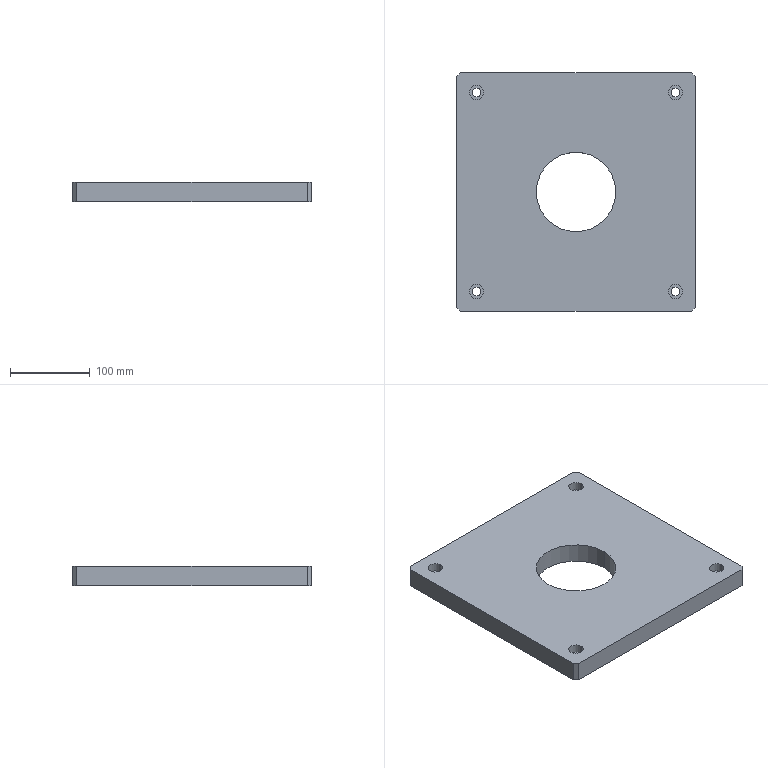Part | STEP file | Backup 2012-3-22-016 | 1 solid | 32 faces | box 300 x 300 x 25 mm | volume 2035882 mm3 | cylinder 18 | plane 14 | commonest cylinder face diameters 11 x8 18 x8 100 x2